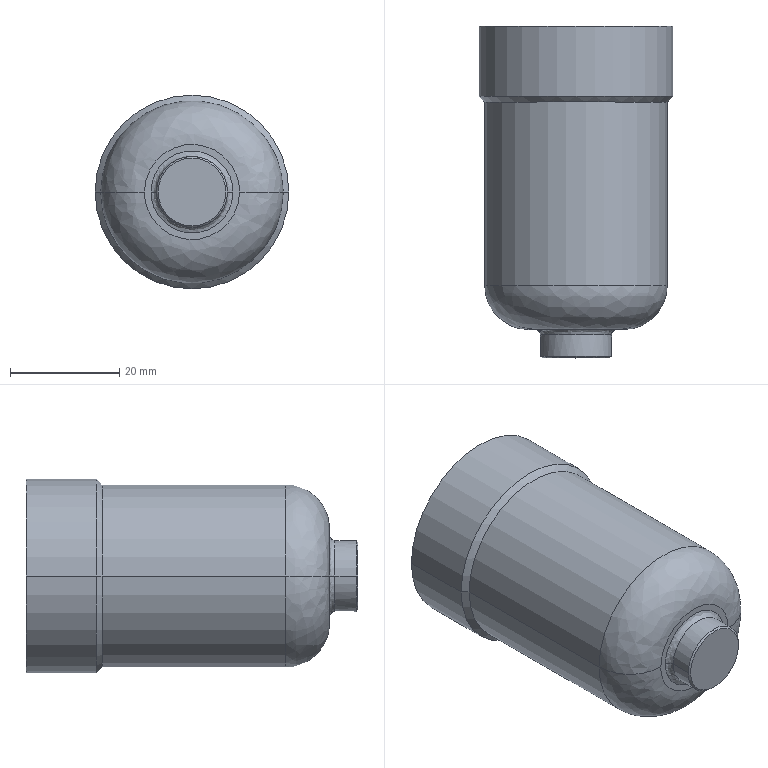Part | SolidWorks | features BaseBody 1 | 1 solid | 26 faces | box 35.465 x 60.7 x 35.465 mm | volume 13088 mm3 | cylinder 10 | cone 6 | spline 4 | plane 4 | torus 2 | commonest cylinder face diameters 13 x2 29.4 x2 31.465 x2 33.4 x2 35.465 x2
STEP:
#1=CARTESIAN_POINT('',(16.7,-47.5,0.));
#2=VERTEX_POINT('',#1);
#3=CARTESIAN_POINT('',(-16.7,-47.5,0.));
#4=VERTEX_POINT('',#3);
#5=CARTESIAN_POINT('',(0.,-47.5,0.));
#6=DIRECTION('',(0.,1.,0.));
#7=DIRECTION('',(1.,0.,0.));
#8=AXIS2_PLACEMENT_3D('',#5,#6,#7);
#9=CIRCLE('',#8,16.7);
#10=EDGE_CURVE('',#2,#4,#9,.T.);
#11=ORIENTED_EDGE('',*,*,#10,.F.);
#12=CARTESIAN_POINT('',(8.7,-55.5,0.));
#13=VERTEX_POINT('',#12);
#14=CARTESIAN_POINT('',(8.7,-47.5,0.));
#15=DIRECTION('',(0.,0.,-1.));
#16=DIRECTION('',(1.,0.,0.));
#17=AXIS2_PLACEMENT_3D('',#14,#15,#16);
#18=CIRCLE('',#17,8.);
#19=EDGE_CURVE('',#2,#13,#18,.T.);
#20=ORIENTED_EDGE('',*,*,#19,.T.);
#21=CARTESIAN_POINT('',(-8.7,-55.5,0.));
#22=VERTEX_POINT('',#21);
#23=CARTESIAN_POINT('',(8.7,-55.5,0.));
#24=CARTESIAN_POINT('',(8.7,-55.5,-17.4));
#25=CARTESIAN_POINT('',(-8.7,-55.5,-17.4));
#26=CARTESIAN_POINT('',(-8.7,-55.5,0.));
#27=(BOUNDED_CURVE()B_SPLINE_CURVE(3,(#23,#24,#25,#26),.UNSPECIFIED.,.F.,.F.)B_SPLINE_CURVE_WITH_KNOTS((4,4),(0.5,1.),.UNSPECIFIED.)CURVE()GEOMETRIC_REPRESENTATION_ITEM()RATIONAL_B_SPLINE_CURVE((1.,0.3333,0.3333,1.))REPRESENTATION_ITEM(''));
#28=EDGE_CURVE('',#13,#22,#27,.T.);
#29=ORIENTED_EDGE('',*,*,#28,.T.);
#30=CARTESIAN_POINT('',(-8.7,-47.5,0.));
#31=DIRECTION('',(0.,0.,1.));
#32=DIRECTION('',(-1.,0.,0.));
#33=AXIS2_PLACEMENT_3D('',#30,#31,#32);
#34=CIRCLE('',#33,8.);
#35=EDGE_CURVE('',#4,#22,#34,.T.);
#36=ORIENTED_EDGE('',*,*,#35,.F.);
#37=EDGE_LOOP('',(#11,#20,#29,#36));
#38=FACE_OUTER_BOUND('',#37,.T.);
#39=CARTESIAN_POINT('',(16.7,-47.5,0.));
#40=CARTESIAN_POINT('',(16.7,-47.5,-33.4));
#41=CARTESIAN_POINT('',(-16.7,-47.5,-33.4));
#42=CARTESIAN_POINT('',(-16.7,-47.5,0.));
#43=CARTESIAN_POINT('',(16.7,-52.186,0.));
#44=CARTESIAN_POINT('',(16.7,-52.186,-33.4));
#45=CARTESIAN_POINT('',(-16.7,-52.186,-33.4));
#46=CARTESIAN_POINT('',(-16.7,-52.186,0.));
#47=CARTESIAN_POINT('',(13.386,-55.5,0.));
#48=CARTESIAN_POINT('',(13.386,-55.5,-26.773));
#49=CARTESIAN_POINT('',(-13.386,-55.5,-26.773));
#50=CARTESIAN_POINT('',(-13.386,-55.5,0.));
#51=CARTESIAN_POINT('',(8.7,-55.5,0.));
#52=CARTESIAN_POINT('',(8.7,-55.5,-17.4));
#53=CARTESIAN_POINT('',(-8.7,-55.5,-17.4));
#54=CARTESIAN_POINT('',(-8.7,-55.5,0.));
#55=(BOUNDED_SURFACE()B_SPLINE_SURFACE(3,3,((#39,#40,#41,#42),(#43,#44,#45,#46),(#47,#48,#49,#50),(#51,#52,#53,#54)),.UNSPECIFIED.,.F.,.F.,.F.)B_SPLINE_SURFACE_WITH_KNOTS((4,4),(4,4),(0.,1.),(0.,1.),.UNSPECIFIED.)GEOMETRIC_REPRESENTATION_ITEM()RATIONAL_B_SPLINE_SURFACE(((1.,0.3333,0.3333,1.),(0.8047,0.2682,0.2682,0.8047),(0.8047,0.2682,0.2682,0.8047),(1.,0.3333,0.3333,1.)))REPRESENTATION_ITEM('')SURFACE());
#56=ADVANCED_FACE('',(#38),#55,.T.);
#57=CARTESIAN_POINT('',(6.5,-56.5,0.));
#58=VERTEX_POINT('',#57);
#59=CARTESIAN_POINT('',(-6.5,-56.5,0.));
#60=VERTEX_POINT('',#59);
#61=CARTESIAN_POINT('',(0.,-56.5,0.));
#62=DIRECTION('',(0.,-1.,0.));
#63=DIRECTION('',(-1.,0.,0.));
#64=AXIS2_PLACEMENT_3D('',#61,#62,#63);
#65=CIRCLE('',#64,6.5);
#66=EDGE_CURVE('',#58,#60,#65,.T.);
#67=ORIENTED_EDGE('',*,*,#66,.F.);
#68=CARTESIAN_POINT('',(7.5,-55.5,0.));
#69=VERTEX_POINT('',#68);
#70=CARTESIAN_POINT('',(7.5,-56.5,0.));
#71=DIRECTION('',(0.,0.,-1.));
#72=DIRECTION('',(1.,0.,0.));
#73=AXIS2_PLACEMENT_3D('',#70,#71,#72);
#74=CIRCLE('',#73,1.);
#75=EDGE_CURVE('',#58,#69,#74,.T.);
#76=ORIENTED_EDGE('',*,*,#75,.T.);
#77=CARTESIAN_POINT('',(-7.5,-55.5,0.));
#78=VERTEX_POINT('',#77);
#79=CARTESIAN_POINT('',(7.5,-55.5,0.));
#80=CARTESIAN_POINT('',(7.5,-55.5,15.));
#81=CARTESIAN_POINT('',(-7.5,-55.5,15.));
#82=CARTESIAN_POINT('',(-7.5,-55.5,0.));
#83=(BOUNDED_CURVE()B_SPLINE_CURVE(3,(#79,#80,#81,#82),.UNSPECIFIED.,.F.,.F.)B_SPLINE_CURVE_WITH_KNOTS((4,4),(0.5,1.),.UNSPECIFIED.)CURVE()GEOMETRIC_REPRESENTATION_ITEM()RATIONAL_B_SPLINE_CURVE((1.,0.3333,0.3333,1.))REPRESENTATION_ITEM(''));
#84=EDGE_CURVE('',#69,#78,#83,.T.);
#85=ORIENTED_EDGE('',*,*,#84,.T.);
#86=CARTESIAN_POINT('',(-7.5,-56.5,0.));
#87=DIRECTION('',(0.,0.,1.));
#88=DIRECTION('',(-1.,0.,0.));
#89=AXIS2_PLACEMENT_3D('',#86,#87,#88);
#90=CIRCLE('',#89,1.);
#91=EDGE_CURVE('',#60,#78,#90,.T.);
#92=ORIENTED_EDGE('',*,*,#91,.F.);
#93=EDGE_LOOP('',(#67,#76,#85,#92));
#94=FACE_OUTER_BOUND('',#93,.T.);
#95=CARTESIAN_POINT('',(-6.5,-56.5,0.));
#96=CARTESIAN_POINT('',(-6.5,-56.5,13.));
#97=CARTESIAN_POINT('',(6.5,-56.5,13.));
#98=CARTESIAN_POINT('',(6.5,-56.5,0.));
#99=CARTESIAN_POINT('',(-6.5,-55.914,0.));
#100=CARTESIAN_POINT('',(-6.5,-55.914,13.));
#101=CARTESIAN_POINT('',(6.5,-55.914,13.));
#102=CARTESIAN_POINT('',(6.5,-55.914,0.));
#103=CARTESIAN_POINT('',(-6.914,-55.5,0.));
#104=CARTESIAN_POINT('',(-6.914,-55.5,13.828));
#105=CARTESIAN_POINT('',(6.914,-55.5,13.828));
#106=CARTESIAN_POINT('',(6.914,-55.5,0.));
#107=CARTESIAN_POINT('',(-7.5,-55.5,0.));
#108=CARTESIAN_POINT('',(-7.5,-55.5,15.));
#109=CARTESIAN_POINT('',(7.5,-55.5,15.));
#110=CARTESIAN_POINT('',(7.5,-55.5,0.));
#111=(BOUNDED_SURFACE()B_SPLINE_SURFACE(3,3,((#95,#96,#97,#98),(#99,#100,#101,#102),(#103,#104,#105,#106),(#107,#108,#109,#110)),.UNSPECIFIED.,.F.,.F.,.F.)B_SPLINE_SURFACE_WITH_KNOTS((4,4),(4,4),(0.,1.),(0.,1.),.UNSPECIFIED.)GEOMETRIC_REPRESENTATION_ITEM()RATIONAL_B_SPLINE_SURFACE(((1.,0.3333,0.3333,1.),(0.8047,0.2682,0.2682,0.8047),(0.8047,0.2682,0.2682,0.8047),(1.,0.3333,0.3333,1.)))REPRESENTATION_ITEM('')SURFACE());
#112=ADVANCED_FACE('',(#94),#111,.F.);
#113=CARTESIAN_POINT('',(16.7,-13.9,0.));
#114=VERTEX_POINT('',#113);
#115=CARTESIAN_POINT('',(-16.7,-13.9,0.));
#116=VERTEX_POINT('',#115);
#117=CARTESIAN_POINT('',(0.,-13.9,0.));
#118=DIRECTION('',(0.,-1.,0.));
#119=DIRECTION('',(1.,0.,0.));
#120=AXIS2_PLACEMENT_3D('',#117,#118,#119);
#121=CIRCLE('',#120,16.7);
#122=EDGE_CURVE('',#114,#116,#121,.T.);
#123=ORIENTED_EDGE('',*,*,#122,.T.);
#124=CARTESIAN_POINT('',(-16.7,0.,0.));
#125=DIRECTION('',(0.,-1.,0.));
#126=VECTOR('',#125,1000.);
#127=LINE('',#124,#126);
#128=EDGE_CURVE('',#116,#4,#127,.T.);
#129=ORIENTED_EDGE('',*,*,#128,.T.);
#130=CARTESIAN_POINT('',(0.,-47.5,0.));
#131=DIRECTION('',(0.,1.,0.));
#132=DIRECTION('',(1.,0.,0.));
#133=AXIS2_PLACEMENT_3D('',#130,#131,#132);
#134=CIRCLE('',#133,16.7);
#135=EDGE_CURVE('',#4,#2,#134,.T.);
#136=ORIENTED_EDGE('',*,*,#135,.T.);
#137=CARTESIAN_POINT('',(16.7,0.,0.));
#138=DIRECTION('',(0.,-1.,0.));
#139=VECTOR('',#138,1000.);
#140=LINE('',#137,#139);
#141=EDGE_CURVE('',#114,#2,#140,.T.);
#142=ORIENTED_EDGE('',*,*,#141,.F.);
#143=EDGE_LOOP('',(#123,#129,#136,#142));
#144=FACE_OUTER_BOUND('',#143,.T.);
#145=CARTESIAN_POINT('',(0.,0.,0.));
#146=DIRECTION('',(0.,-1.,0.));
#147=DIRECTION('',(1.,0.,0.));
#148=AXIS2_PLACEMENT_3D('',#145,#146,#147);
#149=CYLINDRICAL_SURFACE('',#148,16.7);
#150=ADVANCED_FACE('',(#144),#149,.T.);
#151=ORIENTED_EDGE('',*,*,#122,.F.);
#152=CARTESIAN_POINT('',(17.733,-12.867,0.));
#153=VERTEX_POINT('',#152);
#154=CARTESIAN_POINT('',(17.733,-12.867,0.));
#155=DIRECTION('',(0.7071,0.7071,0.));
#156=VECTOR('',#155,1000.);
#157=LINE('',#154,#156);
#158=EDGE_CURVE('',#114,#153,#157,.T.);
#159=ORIENTED_EDGE('',*,*,#158,.T.);
#160=CARTESIAN_POINT('',(-17.732,-12.867,0.));
#161=VERTEX_POINT('',#160);
#162=CARTESIAN_POINT('',(0.,-12.867,0.));
#163=DIRECTION('',(0.,-1.,0.));
#164=DIRECTION('',(-1.,0.,0.));
#165=AXIS2_PLACEMENT_3D('',#162,#163,#164);
#166=CIRCLE('',#165,17.733);
#167=EDGE_CURVE('',#153,#161,#166,.T.);
#168=ORIENTED_EDGE('',*,*,#167,.T.);
#169=CARTESIAN_POINT('',(-17.732,-12.867,0.));
#170=DIRECTION('',(-0.7071,0.7071,0.));
#171=VECTOR('',#170,1000.);
#172=LINE('',#169,#171);
#173=EDGE_CURVE('',#116,#161,#172,.T.);
#174=ORIENTED_EDGE('',*,*,#173,.F.);
#175=EDGE_LOOP('',(#151,#159,#168,#174));
#176=FACE_OUTER_BOUND('',#175,.T.);
#177=CARTESIAN_POINT('',(0.,-12.867,0.));
#178=DIRECTION('',(0.,1.,0.));
#179=DIRECTION('',(-1.,0.,0.));
#180=AXIS2_PLACEMENT_3D('',#177,#178,#179);
#181=CONICAL_SURFACE('',#180,17.733,0.7854);
#182=ADVANCED_FACE('',(#176),#181,.T.);
#183=CARTESIAN_POINT('',(17.733,0.,0.));
#184=VERTEX_POINT('',#183);
#185=CARTESIAN_POINT('',(-17.732,0.,0.));
#186=VERTEX_POINT('',#185);
#187=CARTESIAN_POINT('',(0.,0.,0.));
#188=DIRECTION('',(0.,-1.,0.));
#189=DIRECTION('',(1.,0.,0.));
#190=AXIS2_PLACEMENT_3D('',#187,#188,#189);
#191=CIRCLE('',#190,17.733);
#192=EDGE_CURVE('',#184,#186,#191,.T.);
#193=ORIENTED_EDGE('',*,*,#192,.T.);
#194=CARTESIAN_POINT('',(-17.732,0.,0.));
#195=DIRECTION('',(0.,-1.,0.));
#196=VECTOR('',#195,1000.);
#197=LINE('',#194,#196);
#198=EDGE_CURVE('',#186,#161,#197,.T.);
#199=ORIENTED_EDGE('',*,*,#198,.T.);
#200=ORIENTED_EDGE('',*,*,#167,.F.);
#201=CARTESIAN_POINT('',(17.733,0.,0.));
#202=DIRECTION('',(0.,-1.,0.));
#203=VECTOR('',#202,1000.);
#204=LINE('',#201,#203);
#205=EDGE_CURVE('',#184,#153,#204,.T.);
#206=ORIENTED_EDGE('',*,*,#205,.F.);
#207=EDGE_LOOP('',(#193,#199,#200,#206));
#208=FACE_OUTER_BOUND('',#207,.T.);
#209=CARTESIAN_POINT('',(0.,0.,0.));
#210=DIRECTION('',(0.,-1.,0.));
#211=DIRECTION('',(1.,0.,0.));
#212=AXIS2_PLACEMENT_3D('',#209,#210,#211);
#213=CYLINDRICAL_SURFACE('',#212,17.733);
#214=ADVANCED_FACE('',(#208),#213,.T.);
#215=ORIENTED_EDGE('',*,*,#66,.T.);
#216=CARTESIAN_POINT('',(-6.5,-60.4,0.));
#217=VERTEX_POINT('',#216);
#218=CARTESIAN_POINT('',(-6.5,0.,0.));
#219=DIRECTION('',(0.,-1.,0.));
#220=VECTOR('',#219,1000.);
#221=LINE('',#218,#220);
#222=EDGE_CURVE('',#60,#217,#221,.T.);
#223=ORIENTED_EDGE('',*,*,#222,.T.);
#224=CARTESIAN_POINT('',(0.,-60.4,6.5));
#225=VERTEX_POINT('',#224);
#226=CARTESIAN_POINT('',(0.,-60.4,0.));
#227=DIRECTION('',(0.,1.,0.));
#228=DIRECTION('',(1.,0.,0.));
#229=AXIS2_PLACEMENT_3D('',#226,#227,#228);
#230=CIRCLE('',#229,6.5);
#231=EDGE_CURVE('',#217,#225,#230,.T.);
#232=ORIENTED_EDGE('',*,*,#231,.T.);
#233=CARTESIAN_POINT('',(6.5,-60.4,0.));
#234=VERTEX_POINT('',#233);
#235=CARTESIAN_POINT('',(0.,-60.4,0.));
#236=DIRECTION('',(0.,1.,0.));
#237=DIRECTION('',(1.,0.,0.));
#238=AXIS2_PLACEMENT_3D('',#235,#236,#237);
#239=CIRCLE('',#238,6.5);
#240=EDGE_CURVE('',#225,#234,#239,.T.);
#241=ORIENTED_EDGE('',*,*,#240,.T.);
#242=CARTESIAN_POINT('',(6.5,0.,0.));
#243=DIRECTION('',(0.,-1.,0.));
#244=VECTOR('',#243,1000.);
#245=LINE('',#242,#244);
#246=EDGE_CURVE('',#58,#234,#245,.T.);
#247=ORIENTED_EDGE('',*,*,#246,.F.);
#248=EDGE_LOOP('',(#215,#223,#232,#241,#247));
#249=FACE_OUTER_BOUND('',#248,.T.);
#250=CARTESIAN_POINT('',(0.,0.,0.));
#251=DIRECTION('',(0.,-1.,0.));
#252=DIRECTION('',(1.,0.,0.));
#253=AXIS2_PLACEMENT_3D('',#250,#251,#252);
#254=CYLINDRICAL_SURFACE('',#253,6.5);
#255=ADVANCED_FACE('',(#249),#254,.T.);
#256=CARTESIAN_POINT('',(15.733,0.,0.));
#257=VERTEX_POINT('',#256);
#258=CARTESIAN_POINT('',(-15.732,0.,0.));
#259=VERTEX_POINT('',#258);
#260=CARTESIAN_POINT('',(0.,0.,0.));
#261=DIRECTION('',(0.,1.,0.));
#262=DIRECTION('',(1.,0.,0.));
#263=AXIS2_PLACEMENT_3D('',#260,#261,#262);
#264=CIRCLE('',#263,15.732);
#265=EDGE_CURVE('',#257,#259,#264,.T.);
#266=ORIENTED_EDGE('',*,*,#265,.T.);
#267=CARTESIAN_POINT('',(-15.732,-12.039,0.));
#268=VERTEX_POINT('',#267);
#269=CARTESIAN_POINT('',(-15.732,0.,0.));
#270=DIRECTION('',(0.,-1.,0.));
#271=VECTOR('',#270,1000.);
#272=LINE('',#269,#271);
#273=EDGE_CURVE('',#259,#268,#272,.T.);
#274=ORIENTED_EDGE('',*,*,#273,.T.);
#275=CARTESIAN_POINT('',(15.733,-12.039,0.));
#276=VERTEX_POINT('',#275);
#277=CARTESIAN_POINT('',(0.,-12.039,0.));
#278=DIRECTION('',(0.,1.,0.));
#279=DIRECTION('',(1.,0.,0.));
#280=AXIS2_PLACEMENT_3D('',#277,#278,#279);
#281=CIRCLE('',#280,15.732);
#282=EDGE_CURVE('',#276,#268,#281,.T.);
#283=ORIENTED_EDGE('',*,*,#282,.F.);
#284=CARTESIAN_POINT('',(15.733,0.,0.));
#285=DIRECTION('',(0.,-1.,0.));
#286=VECTOR('',#285,1000.);
#287=LINE('',#284,#286);
#288=EDGE_CURVE('',#257,#276,#287,.T.);
#289=ORIENTED_EDGE('',*,*,#288,.F.);
#290=EDGE_LOOP('',(#266,#274,#283,#289));
#291=FACE_OUTER_BOUND('',#290,.T.);
#292=CARTESIAN_POINT('',(0.,0.,0.));
#293=DIRECTION('',(0.,-1.,0.));
#294=DIRECTION('',(1.,0.,0.));
#295=AXIS2_PLACEMENT_3D('',#292,#293,#294);
#296=CYLINDRICAL_SURFACE('',#295,15.732);
#297=ADVANCED_FACE('',(#291),#296,.F.);
#298=CARTESIAN_POINT('',(0.,-60.7,6.2));
#299=VERTEX_POINT('',#298);
#300=CARTESIAN_POINT('',(0.,-60.7,-6.2));
#301=VERTEX_POINT('',#300);
#302=CARTESIAN_POINT('',(0.,-60.7,0.));
#303=DIRECTION('',(0.,1.,0.));
#304=DIRECTION('',(0.,0.,1.));
#305=AXIS2_PLACEMENT_3D('',#302,#303,#304);
#306=CIRCLE('',#305,6.2);
#307=EDGE_CURVE('',#299,#301,#306,.T.);
#308=ORIENTED_EDGE('',*,*,#307,.T.);
#309=CARTESIAN_POINT('',(0.,-60.4,-6.5));
#310=VERTEX_POINT('',#309);
#311=CARTESIAN_POINT('',(0.,-60.4,-6.5));
#312=DIRECTION('',(0.,0.7071,-0.7071));
#313=VECTOR('',#312,1000.);
#314=LINE('',#311,#313);
#315=EDGE_CURVE('',#301,#310,#314,.T.);
#316=ORIENTED_EDGE('',*,*,#315,.T.);
#317=CARTESIAN_POINT('',(0.,-60.4,0.));
#318=DIRECTION('',(0.,1.,0.));
#319=DIRECTION('',(1.,0.,0.));
#320=AXIS2_PLACEMENT_3D('',#317,#318,#319);
#321=CIRCLE('',#320,6.5);
#322=EDGE_CURVE('',#234,#310,#321,.T.);
#323=ORIENTED_EDGE('',*,*,#322,.F.);
#324=ORIENTED_EDGE('',*,*,#240,.F.);
#325=CARTESIAN_POINT('',(0.,-60.4,6.5));
#326=DIRECTION('',(0.,0.7071,0.7071));
#327=VECTOR('',#326,1000.);
#328=LINE('',#325,#327);
#329=EDGE_CURVE('',#299,#225,#328,.T.);
#330=ORIENTED_EDGE('',*,*,#329,.F.);
#331=EDGE_LOOP('',(#308,#316,#323,#324,#330));
#332=FACE_OUTER_BOUND('',#331,.T.);
#333=CARTESIAN_POINT('',(0.,-60.4,0.));
#334=DIRECTION('',(0.,1.,0.));
#335=DIRECTION('',(0.,0.,1.));
#336=AXIS2_PLACEMENT_3D('',#333,#334,#335);
#337=CONICAL_SURFACE('',#336,6.5,0.7854);
#338=ADVANCED_FACE('',(#332),#337,.T.);
#339=CARTESIAN_POINT('',(14.7,-13.072,0.));
#340=VERTEX_POINT('',#339);
#341=CARTESIAN_POINT('',(-14.7,-13.072,0.));
#342=VERTEX_POINT('',#341);
#343=CARTESIAN_POINT('',(0.,-13.072,0.));
#344=DIRECTION('',(0.,1.,0.));
#345=DIRECTION('',(-1.,0.,0.));
#346=AXIS2_PLACEMENT_3D('',#343,#344,#345);
#347=CIRCLE('',#346,14.7);
#348=EDGE_CURVE('',#340,#342,#347,.T.);
#349=ORIENTED_EDGE('',*,*,#348,.F.);
#350=CARTESIAN_POINT('',(15.733,-12.039,0.));
#351=DIRECTION('',(0.7071,0.7071,0.));
#352=VECTOR('',#351,1000.);
#353=LINE('',#350,#352);
#354=EDGE_CURVE('',#340,#276,#353,.T.);
#355=ORIENTED_EDGE('',*,*,#354,.T.);
#356=ORIENTED_EDGE('',*,*,#282,.T.);
#357=CARTESIAN_POINT('',(-15.732,-12.039,0.));
#358=DIRECTION('',(-0.7071,0.7071,0.));
#359=VECTOR('',#358,1000.);
#360=LINE('',#357,#359);
#361=EDGE_CURVE('',#342,#268,#360,.T.);
#362=ORIENTED_EDGE('',*,*,#361,.F.);
#363=EDGE_LOOP('',(#349,#355,#356,#362));
#364=FACE_OUTER_BOUND('',#363,.T.);
#365=CARTESIAN_POINT('',(0.,-12.039,0.));
#366=DIRECTION('',(0.,1.,0.));
#367=DIRECTION('',(-1.,0.,0.));
#368=AXIS2_PLACEMENT_3D('',#365,#366,#367);
#369=CONICAL_SURFACE('',#368,15.733,0.7854);
#370=ADVANCED_FACE('',(#364),#369,.F.);
#371=ORIENTED_EDGE('',*,*,#348,.T.);
#372=CARTESIAN_POINT('',(-14.7,-45.5,0.));
#373=VERTEX_POINT('',#372);
#374=CARTESIAN_POINT('',(-14.7,0.,0.));
#375=DIRECTION('',(0.,-1.,0.));
#376=VECTOR('',#375,1000.);
#377=LINE('',#374,#376);
#378=EDGE_CURVE('',#342,#373,#377,.T.);
#379=ORIENTED_EDGE('',*,*,#378,.T.);
#380=CARTESIAN_POINT('',(0.,-45.5,-14.7));
#381=VERTEX_POINT('',#380);
#382=CARTESIAN_POINT('',(0.,-45.5,0.));
#383=DIRECTION('',(0.,1.,0.));
#384=DIRECTION('',(1.,0.,0.));
#385=AXIS2_PLACEMENT_3D('',#382,#383,#384);
#386=CIRCLE('',#385,14.7);
#387=EDGE_CURVE('',#381,#373,#386,.T.);
#388=ORIENTED_EDGE('',*,*,#387,.F.);
#389=CARTESIAN_POINT('',(14.7,-45.5,0.));
#390=VERTEX_POINT('',#389);
#391=CARTESIAN_POINT('',(0.,-45.5,0.));
#392=DIRECTION('',(0.,1.,0.));
#393=DIRECTION('',(1.,0.,0.));
#394=AXIS2_PLACEMENT_3D('',#391,#392,#393);
#395=CIRCLE('',#394,14.7);
#396=EDGE_CURVE('',#390,#381,#395,.T.);
#397=ORIENTED_EDGE('',*,*,#396,.F.);
#398=CARTESIAN_POINT('',(14.7,0.,0.));
#399=DIRECTION('',(0.,-1.,0.));
#400=VECTOR('',#399,1000.);
#401=LINE('',#398,#400);
#402=EDGE_CURVE('',#340,#390,#401,.T.);
#403=ORIENTED_EDGE('',*,*,#402,.F.);
#404=EDGE_LOOP('',(#371,#379,#388,#397,#403));
#405=FACE_OUTER_BOUND('',#404,.T.);
#406=CARTESIAN_POINT('',(0.,0.,0.));
#407=DIRECTION('',(0.,-1.,0.));
#408=DIRECTION('',(1.,0.,0.));
#409=AXIS2_PLACEMENT_3D('',#406,#407,#408);
#410=CYLINDRICAL_SURFACE('',#409,14.7);
#411=ADVANCED_FACE('',(#405),#410,.F.);
#412=CARTESIAN_POINT('',(0.,-53.5,-6.7));
#413=VERTEX_POINT('',#412);
#414=CARTESIAN_POINT('',(0.,-53.5,6.7));
#415=VERTEX_POINT('',#414);
#416=CARTESIAN_POINT('',(0.,-53.5,0.));
#417=DIRECTION('',(0.,1.,0.));
#418=DIRECTION('',(0.,0.,1.));
#419=AXIS2_PLACEMENT_3D('',#416,#417,#418);
#420=CIRCLE('',#419,6.7);
#421=EDGE_CURVE('',#413,#415,#420,.T.);
#422=ORIENTED_EDGE('',*,*,#421,.F.);
#423=CARTESIAN_POINT('',(0.,-45.5,-6.7));
#424=DIRECTION('',(1.,0.,0.));
#425=DIRECTION('',(0.,0.,-1.));
#426=AXIS2_PLACEMENT_3D('',#423,#424,#425);
#427=CIRCLE('',#426,8.);
#428=EDGE_CURVE('',#413,#381,#427,.T.);
#429=ORIENTED_EDGE('',*,*,#428,.T.);
#430=ORIENTED_EDGE('',*,*,#387,.T.);
#431=CARTESIAN_POINT('',(0.,-45.5,14.7));
#432=VERTEX_POINT('',#431);
#433=CARTESIAN_POINT('',(0.,-45.5,0.));
#434=DIRECTION('',(0.,1.,0.));
#435=DIRECTION('',(1.,0.,0.));
#436=AXIS2_PLACEMENT_3D('',#433,#434,#435);
#437=CIRCLE('',#436,14.7);
#438=EDGE_CURVE('',#373,#432,#437,.T.);
#439=ORIENTED_EDGE('',*,*,#438,.T.);
#440=CARTESIAN_POINT('',(0.,-45.5,6.7));
#441=DIRECTION('',(-1.,0.,0.));
#442=DIRECTION('',(0.,0.,1.));
#443=AXIS2_PLACEMENT_3D('',#440,#441,#442);
#444=CIRCLE('',#443,8.);
#445=EDGE_CURVE('',#415,#432,#444,.T.);
#446=ORIENTED_EDGE('',*,*,#445,.F.);
#447=EDGE_LOOP('',(#422,#429,#430,#439,#446));
#448=FACE_OUTER_BOUND('',#447,.T.);
#449=CARTESIAN_POINT('',(0.,-45.5,0.));
#450=DIRECTION('',(0.,1.,0.));
#451=DIRECTION('',(0.,0.,1.));
#452=AXIS2_PLACEMENT_3D('',#449,#450,#451);
#453=TOROIDAL_SURFACE('',#452,6.7,8.);
#454=ADVANCED_FACE('',(#448),#453,.F.);
#455=ORIENTED_EDGE('',*,*,#128,.F.);
#456=CARTESIAN_POINT('',(0.,-13.9,0.));
#457=DIRECTION('',(0.,-1.,0.));
#458=DIRECTION('',(1.,0.,0.));
#459=AXIS2_PLACEMENT_3D('',#456,#457,#458);
#460=CIRCLE('',#459,16.7);
#461=EDGE_CURVE('',#116,#114,#460,.T.);
#462=ORIENTED_EDGE('',*,*,#461,.T.);
#463=ORIENTED_EDGE('',*,*,#141,.T.);
#464=ORIENTED_EDGE('',*,*,#10,.T.);
#465=EDGE_LOOP('',(#455,#462,#463,#464));
#466=FACE_OUTER_BOUND('',#465,.T.);
#467=CARTESIAN_POINT('',(0.,0.,0.));
#468=DIRECTION('',(0.,-1.,0.));
#469=DIRECTION('',(1.,0.,0.));
#470=AXIS2_PLACEMENT_3D('',#467,#468,#469);
#471=CYLINDRICAL_SURFACE('',#470,16.7);
#472=ADVANCED_FACE('',(#466),#471,.T.);
#473=ORIENTED_EDGE('',*,*,#19,.F.);
#474=ORIENTED_EDGE('',*,*,#135,.F.);
#475=ORIENTED_EDGE('',*,*,#35,.T.);
#476=CARTESIAN_POINT('',(-8.7,-55.5,0.));
#477=CARTESIAN_POINT('',(-8.7,-55.5,17.4));
#478=CARTESIAN_POINT('',(8.7,-55.5,17.4));
#479=CARTESIAN_POINT('',(8.7,-55.5,0.));
#480=(BOUNDED_CURVE()B_SPLINE_CURVE(3,(#476,#477,#478,#479),.UNSPECIFIED.,.F.,.F.)B_SPLINE_CURVE_WITH_KNOTS((4,4),(0.,0.5),.UNSPECIFIED.)CURVE()GEOMETRIC_REPRESENTATION_ITEM()RATIONAL_B_SPLINE_CURVE((1.,0.3333,0.3333,1.))REPRESENTATION_ITEM(''));
#481=EDGE_CURVE('',#22,#13,#480,.T.);
#482=ORIENTED_EDGE('',*,*,#481,.T.);
#483=EDGE_LOOP('',(#473,#474,#475,#482));
#484=FACE_OUTER_BOUND('',#483,.T.);
#485=CARTESIAN_POINT('',(-16.7,-47.5,0.));
#486=CARTESIAN_POINT('',(-16.7,-47.5,33.4));
#487=CARTESIAN_POINT('',(16.7,-47.5,33.4));
#488=CARTESIAN_POINT('',(16.7,-47.5,0.));
#489=CARTESIAN_POINT('',(-16.7,-52.186,0.));
#490=CARTESIAN_POINT('',(-16.7,-52.186,33.4));
#491=CARTESIAN_POINT('',(16.7,-52.186,33.4));
#492=CARTESIAN_POINT('',(16.7,-52.186,0.));
#493=CARTESIAN_POINT('',(-13.386,-55.5,0.));
#494=CARTESIAN_POINT('',(-13.386,-55.5,26.773));
#495=CARTESIAN_POINT('',(13.386,-55.5,26.773));
#496=CARTESIAN_POINT('',(13.386,-55.5,0.));
#497=CARTESIAN_POINT('',(-8.7,-55.5,0.));
#498=CARTESIAN_POINT('',(-8.7,-55.5,17.4));
#499=CARTESIAN_POINT('',(8.7,-55.5,17.4));
#500=CARTESIAN_POINT('',(8.7,-55.5,0.));
#501=(BOUNDED_SURFACE()B_SPLINE_SURFACE(3,3,((#485,#486,#487,#488),(#489,#490,#491,#492),(#493,#494,#495,#496),(#497,#498,#499,#500)),.UNSPECIFIED.,.F.,.F.,.F.)B_SPLINE_SURFACE_WITH_KNOTS((4,4),(4,4),(0.,1.),(0.,1.),.UNSPECIFIED.)GEOMETRIC_REPRESENTATION_ITEM()RATIONAL_B_SPLINE_SURFACE(((1.,0.3333,0.3333,1.),(0.8047,0.2682,0.2682,0.8047),(0.8047,0.2682,0.2682,0.8047),(1.,0.3333,0.3333,1.)))REPRESENTATION_ITEM('')SURFACE());
#502=ADVANCED_FACE('',(#484),#501,.T.);
#503=ORIENTED_EDGE('',*,*,#158,.F.);
#504=ORIENTED_EDGE('',*,*,#461,.F.);
#505=ORIENTED_EDGE('',*,*,#173,.T.);
#506=CARTESIAN_POINT('',(0.,-12.867,0.));
#507=DIRECTION('',(0.,-1.,0.));
#508=DIRECTION('',(-1.,0.,0.));
#509=AXIS2_PLACEMENT_3D('',#506,#507,#508);
#510=CIRCLE('',#509,17.733);
#511=EDGE_CURVE('',#161,#153,#510,.T.);
#512=ORIENTED_EDGE('',*,*,#511,.T.);
#513=EDGE_LOOP('',(#503,#504,#505,#512));
#514=FACE_OUTER_BOUND('',#513,.T.);
#515=CARTESIAN_POINT('',(0.,-12.867,0.));
#516=DIRECTION('',(0.,1.,0.));
#517=DIRECTION('',(-1.,0.,0.));
#518=AXIS2_PLACEMENT_3D('',#515,#516,#517);
#519=CONICAL_SURFACE('',#518,17.733,0.7854);
#520=ADVANCED_FACE('',(#514),#519,.T.);
#521=CARTESIAN_POINT('',(-7.5,-55.5,0.));
#522=CARTESIAN_POINT('',(-7.5,-55.5,-15.));
#523=CARTESIAN_POINT('',(7.5,-55.5,-15.));
#524=CARTESIAN_POINT('',(7.5,-55.5,0.));
#525=(BOUNDED_CURVE()B_SPLINE_CURVE(3,(#521,#522,#523,#524),.UNSPECIFIED.,.F.,.F.)B_SPLINE_CURVE_WITH_KNOTS((4,4),(0.,0.5),.UNSPECIFIED.)CURVE()GEOMETRIC_REPRESENTATION_ITEM()RATIONAL_B_SPLINE_CURVE((1.,0.3333,0.3333,1.))REPRESENTATION_ITEM(''));
#526=EDGE_CURVE('',#78,#69,#525,.T.);
#527=ORIENTED_EDGE('',*,*,#526,.F.);
#528=ORIENTED_EDGE('',*,*,#84,.F.);
#529=EDGE_LOOP('',(#527,#528));
#530=FACE_BOUND('',#529,.T.);
#531=ORIENTED_EDGE('',*,*,#481,.F.);
#532=ORIENTED_EDGE('',*,*,#28,.F.);
#533=EDGE_LOOP('',(#531,#532));
#534=FACE_OUTER_BOUND('',#533,.T.);
#535=CARTESIAN_POINT('',(-7.5,-55.5,0.));
#536=DIRECTION('',(0.,1.,0.));
#537=DIRECTION('',(-1.,0.,0.));
#538=AXIS2_PLACEMENT_3D('',#535,#536,#537);
#539=PLANE('',#538);
#540=ADVANCED_FACE('',(#530,#534),#539,.F.);
#541=ORIENTED_EDGE('',*,*,#198,.F.);
#542=CARTESIAN_POINT('',(0.,0.,0.));
#543=DIRECTION('',(0.,-1.,0.));
#544=DIRECTION('',(1.,0.,0.));
#545=AXIS2_PLACEMENT_3D('',#542,#543,#544);
#546=CIRCLE('',#545,17.733);
#547=EDGE_CURVE('',#186,#184,#546,.T.);
#548=ORIENTED_EDGE('',*,*,#547,.T.);
#549=ORIENTED_EDGE('',*,*,#205,.T.);
#550=ORIENTED_EDGE('',*,*,#511,.F.);
#551=EDGE_LOOP('',(#541,#548,#549,#550));
#552=FACE_OUTER_BOUND('',#551,.T.);
#553=CARTESIAN_POINT('',(0.,0.,0.));
#554=DIRECTION('',(0.,-1.,0.));
#555=DIRECTION('',(1.,0.,0.));
#556=AXIS2_PLACEMENT_3D('',#553,#554,#555);
#557=CYLINDRICAL_SURFACE('',#556,17.733);
#558=ADVANCED_FACE('',(#552),#557,.T.);
#559=ORIENTED_EDGE('',*,*,#75,.F.);
#560=CARTESIAN_POINT('',(0.,-56.5,0.));
#561=DIRECTION('',(0.,-1.,0.));
#562=DIRECTION('',(-1.,0.,0.));
#563=AXIS2_PLACEMENT_3D('',#560,#561,#562);
#564=CIRCLE('',#563,6.5);
#565=EDGE_CURVE('',#60,#58,#564,.T.);
#566=ORIENTED_EDGE('',*,*,#565,.F.);
#567=ORIENTED_EDGE('',*,*,#91,.T.);
#568=ORIENTED_EDGE('',*,*,#526,.T.);
#569=EDGE_LOOP('',(#559,#566,#567,#568));
#570=FACE_OUTER_BOUND('',#569,.T.);
#571=CARTESIAN_POINT('',(6.5,-56.5,0.));
#572=CARTESIAN_POINT('',(6.5,-56.5,-13.));
#573=CARTESIAN_POINT('',(-6.5,-56.5,-13.));
#574=CARTESIAN_POINT('',(-6.5,-56.5,0.));
#575=CARTESIAN_POINT('',(6.5,-55.914,0.));
#576=CARTESIAN_POINT('',(6.5,-55.914,-13.));
#577=CARTESIAN_POINT('',(-6.5,-55.914,-13.));
#578=CARTESIAN_POINT('',(-6.5,-55.914,0.));
#579=CARTESIAN_POINT('',(6.914,-55.5,0.));
#580=CARTESIAN_POINT('',(6.914,-55.5,-13.828));
#581=CARTESIAN_POINT('',(-6.914,-55.5,-13.828));
#582=CARTESIAN_POINT('',(-6.914,-55.5,0.));
#583=CARTESIAN_POINT('',(7.5,-55.5,0.));
#584=CARTESIAN_POINT('',(7.5,-55.5,-15.));
#585=CARTESIAN_POINT('',(-7.5,-55.5,-15.));
#586=CARTESIAN_POINT('',(-7.5,-55.5,0.));
#587=(BOUNDED_SURFACE()B_SPLINE_SURFACE(3,3,((#571,#572,#573,#574),(#575,#576,#577,#578),(#579,#580,#581,#582),(#583,#584,#585,#586)),.UNSPECIFIED.,.F.,.F.,.F.)B_SPLINE_SURFACE_WITH_KNOTS((4,4),(4,4),(0.,1.),(0.,1.),.UNSPECIFIED.)GEOMETRIC_REPRESENTATION_ITEM()RATIONAL_B_SPLINE_SURFACE(((1.,0.3333,0.3333,1.),(0.8047,0.2682,0.2682,0.8047),(0.8047,0.2682,0.2682,0.8047),(1.,0.3333,0.3333,1.)))REPRESENTATION_ITEM('')SURFACE());
#588=ADVANCED_FACE('',(#570),#587,.F.);
#589=ORIENTED_EDGE('',*,*,#192,.F.);
#590=ORIENTED_EDGE('',*,*,#547,.F.);
#591=EDGE_LOOP('',(#589,#590));
#592=FACE_OUTER_BOUND('',#591,.T.);
#593=ORIENTED_EDGE('',*,*,#265,.F.);
#594=CARTESIAN_POINT('',(0.,0.,0.));
#595=DIRECTION('',(0.,1.,0.));
#596=DIRECTION('',(1.,0.,0.));
#597=AXIS2_PLACEMENT_3D('',#594,#595,#596);
#598=CIRCLE('',#597,15.732);
#599=EDGE_CURVE('',#259,#257,#598,.T.);
#600=ORIENTED_EDGE('',*,*,#599,.F.);
#601=EDGE_LOOP('',(#593,#600));
#602=FACE_BOUND('',#601,.T.);
#603=CARTESIAN_POINT('',(-17.733,0.,0.));
#604=DIRECTION('',(0.,-1.,0.));
#605=DIRECTION('',(1.,0.,0.));
#606=AXIS2_PLACEMENT_3D('',#603,#604,#605);
#607=PLANE('',#606);
#608=ADVANCED_FACE('',(#592,#602),#607,.F.);
#609=ORIENTED_EDGE('',*,*,#222,.F.);
#610=ORIENTED_EDGE('',*,*,#565,.T.);
#611=ORIENTED_EDGE('',*,*,#246,.T.);
#612=ORIENTED_EDGE('',*,*,#322,.T.);
#613=CARTESIAN_POINT('',(0.,-60.4,0.));
#614=DIRECTION('',(0.,1.,0.));
#615=DIRECTION('',(1.,0.,0.));
#616=AXIS2_PLACEMENT_3D('',#613,#614,#615);
#617=CIRCLE('',#616,6.5);
#618=EDGE_CURVE('',#310,#217,#617,.T.);
#619=ORIENTED_EDGE('',*,*,#618,.T.);
#620=EDGE_LOOP('',(#609,#610,#611,#612,#619));
#621=FACE_OUTER_BOUND('',#620,.T.);
#622=CARTESIAN_POINT('',(0.,0.,0.));
#623=DIRECTION('',(0.,-1.,0.));
#624=DIRECTION('',(1.,0.,0.));
#625=AXIS2_PLACEMENT_3D('',#622,#623,#624);
#626=CYLINDRICAL_SURFACE('',#625,6.5);
#627=ADVANCED_FACE('',(#621),#626,.T.);
#628=ORIENTED_EDGE('',*,*,#273,.F.);
#629=ORIENTED_EDGE('',*,*,#599,.T.);
#630=ORIENTED_EDGE('',*,*,#288,.T.);
#631=CARTESIAN_POINT('',(0.,-12.039,0.));
#632=DIRECTION('',(0.,1.,0.));
#633=DIRECTION('',(1.,0.,0.));
#634=AXIS2_PLACEMENT_3D('',#631,#632,#633);
#635=CIRCLE('',#634,15.732);
#636=EDGE_CURVE('',#268,#276,#635,.T.);
#637=ORIENTED_EDGE('',*,*,#636,.F.);
#638=EDGE_LOOP('',(#628,#629,#630,#637));
#639=FACE_OUTER_BOUND('',#638,.T.);
#640=CARTESIAN_POINT('',(0.,0.,0.));
#641=DIRECTION('',(0.,-1.,0.));
#642=DIRECTION('',(1.,0.,0.));
#643=AXIS2_PLACEMENT_3D('',#640,#641,#642);
#644=CYLINDRICAL_SURFACE('',#643,15.732);
#645=ADVANCED_FACE('',(#639),#644,.F.);
#646=ORIENTED_EDGE('',*,*,#315,.F.);
#647=CARTESIAN_POINT('',(0.,-60.7,0.));
#648=DIRECTION('',(0.,1.,0.));
#649=DIRECTION('',(0.,0.,1.));
#650=AXIS2_PLACEMENT_3D('',#647,#648,#649);
#651=CIRCLE('',#650,6.2);
#652=EDGE_CURVE('',#301,#299,#651,.T.);
#653=ORIENTED_EDGE('',*,*,#652,.T.);
#654=ORIENTED_EDGE('',*,*,#329,.T.);
#655=ORIENTED_EDGE('',*,*,#231,.F.);
#656=ORIENTED_EDGE('',*,*,#618,.F.);
#657=EDGE_LOOP('',(#646,#653,#654,#655,#656));
#658=FACE_OUTER_BOUND('',#657,.T.);
#659=CARTESIAN_POINT('',(0.,-60.4,0.));
#660=DIRECTION('',(0.,1.,0.));
#661=DIRECTION('',(0.,0.,1.));
#662=AXIS2_PLACEMENT_3D('',#659,#660,#661);
#663=CONICAL_SURFACE('',#662,6.5,0.7854);
#664=ADVANCED_FACE('',(#658),#663,.T.);
#665=ORIENTED_EDGE('',*,*,#354,.F.);
#666=CARTESIAN_POINT('',(0.,-13.072,0.));
#667=DIRECTION('',(0.,1.,0.));
#668=DIRECTION('',(-1.,0.,0.));
#669=AXIS2_PLACEMENT_3D('',#666,#667,#668);
#670=CIRCLE('',#669,14.7);
#671=EDGE_CURVE('',#342,#340,#670,.T.);
#672=ORIENTED_EDGE('',*,*,#671,.F.);
#673=ORIENTED_EDGE('',*,*,#361,.T.);
#674=ORIENTED_EDGE('',*,*,#636,.T.);
#675=EDGE_LOOP('',(#665,#672,#673,#674));
#676=FACE_OUTER_BOUND('',#675,.T.);
#677=CARTESIAN_POINT('',(0.,-12.039,0.));
#678=DIRECTION('',(0.,1.,0.));
#679=DIRECTION('',(-1.,0.,0.));
#680=AXIS2_PLACEMENT_3D('',#677,#678,#679);
#681=CONICAL_SURFACE('',#680,15.733,0.7854);
#682=ADVANCED_FACE('',(#676),#681,.F.);
#683=ORIENTED_EDGE('',*,*,#307,.F.);
#684=ORIENTED_EDGE('',*,*,#652,.F.);
#685=EDGE_LOOP('',(#683,#684));
#686=FACE_OUTER_BOUND('',#685,.T.);
#687=CARTESIAN_POINT('',(0.,-60.7,0.));
#688=DIRECTION('',(0.,1.,0.));
#689=DIRECTION('',(-1.,0.,0.));
#690=AXIS2_PLACEMENT_3D('',#687,#688,#689);
#691=PLANE('',#690);
#692=ADVANCED_FACE('',(#686),#691,.F.);
#693=ORIENTED_EDGE('',*,*,#378,.F.);
#694=ORIENTED_EDGE('',*,*,#671,.T.);
#695=ORIENTED_EDGE('',*,*,#402,.T.);
#696=CARTESIAN_POINT('',(0.,-45.5,0.));
#697=DIRECTION('',(0.,1.,0.));
#698=DIRECTION('',(1.,0.,0.));
#699=AXIS2_PLACEMENT_3D('',#696,#697,#698);
#700=CIRCLE('',#699,14.7);
#701=EDGE_CURVE('',#432,#390,#700,.T.);
#702=ORIENTED_EDGE('',*,*,#701,.F.);
#703=ORIENTED_EDGE('',*,*,#438,.F.);
#704=EDGE_LOOP('',(#693,#694,#695,#702,#703));
#705=FACE_OUTER_BOUND('',#704,.T.);
#706=CARTESIAN_POINT('',(0.,0.,0.));
#707=DIRECTION('',(0.,-1.,0.));
#708=DIRECTION('',(1.,0.,0.));
#709=AXIS2_PLACEMENT_3D('',#706,#707,#708);
#710=CYLINDRICAL_SURFACE('',#709,14.7);
#711=ADVANCED_FACE('',(#705),#710,.F.);
#712=ORIENTED_EDGE('',*,*,#428,.F.);
#713=CARTESIAN_POINT('',(0.,-53.5,0.));
#714=DIRECTION('',(0.,1.,0.));
#715=DIRECTION('',(0.,0.,1.));
#716=AXIS2_PLACEMENT_3D('',#713,#714,#715);
#717=CIRCLE('',#716,6.7);
#718=EDGE_CURVE('',#415,#413,#717,.T.);
#719=ORIENTED_EDGE('',*,*,#718,.F.);
#720=ORIENTED_EDGE('',*,*,#445,.T.);
#721=ORIENTED_EDGE('',*,*,#701,.T.);
#722=ORIENTED_EDGE('',*,*,#396,.T.);
#723=EDGE_LOOP('',(#712,#719,#720,#721,#722));
#724=FACE_OUTER_BOUND('',#723,.T.);
#725=CARTESIAN_POINT('',(0.,-45.5,0.));
#726=DIRECTION('',(0.,1.,0.));
#727=DIRECTION('',(0.,0.,1.));
#728=AXIS2_PLACEMENT_3D('',#725,#726,#727);
#729=TOROIDAL_SURFACE('',#728,6.7,8.);
#730=ADVANCED_FACE('',(#724),#729,.F.);
#731=ORIENTED_EDGE('',*,*,#718,.T.);
#732=ORIENTED_EDGE('',*,*,#421,.T.);
#733=EDGE_LOOP('',(#731,#732));
#734=FACE_OUTER_BOUND('',#733,.T.);
#735=CARTESIAN_POINT('',(-6.7,-53.5,0.));
#736=DIRECTION('',(0.,-1.,0.));
#737=DIRECTION('',(1.,0.,0.));
#738=AXIS2_PLACEMENT_3D('',#735,#736,#737);
#739=PLANE('',#738);
#740=ADVANCED_FACE('',(#734),#739,.F.);
#741=CLOSED_SHELL('',(#56,#112,#150,#182,#214,#255,#297,#338,#370,#411,#454,#472,#502,#520,#540,#558,#588,#608,#627,#645,#664,#682,#692,#711,#730,#740));
#742=MANIFOLD_SOLID_BREP('',#741);
#743=CARTESIAN_POINT('',(0.,0.,0.));
#744=DIRECTION('',(0.,0.,1.));
#745=DIRECTION('',(1.,0.,0.));
#746=AXIS2_PLACEMENT_3D('',#743,#744,#745);
#747=(LENGTH_UNIT()NAMED_UNIT(*)SI_UNIT(.MILLI.,.METRE.));
#748=UNCERTAINTY_MEASURE_WITH_UNIT(LENGTH_MEASURE(0.00001),#747,'','');
#749=(NAMED_UNIT(*)PLANE_ANGLE_UNIT()SI_UNIT($,.RADIAN.));
#750=(NAMED_UNIT(*)SI_UNIT($,.STERADIAN.)SOLID_ANGLE_UNIT());
#751=(GEOMETRIC_REPRESENTATION_CONTEXT(3)GLOBAL_UNCERTAINTY_ASSIGNED_CONTEXT((#748))GLOBAL_UNIT_ASSIGNED_CONTEXT((#747,#749,#750))REPRESENTATION_CONTEXT('',''));
#752=ADVANCED_BREP_SHAPE_REPRESENTATION('',(#742,#746),#751);